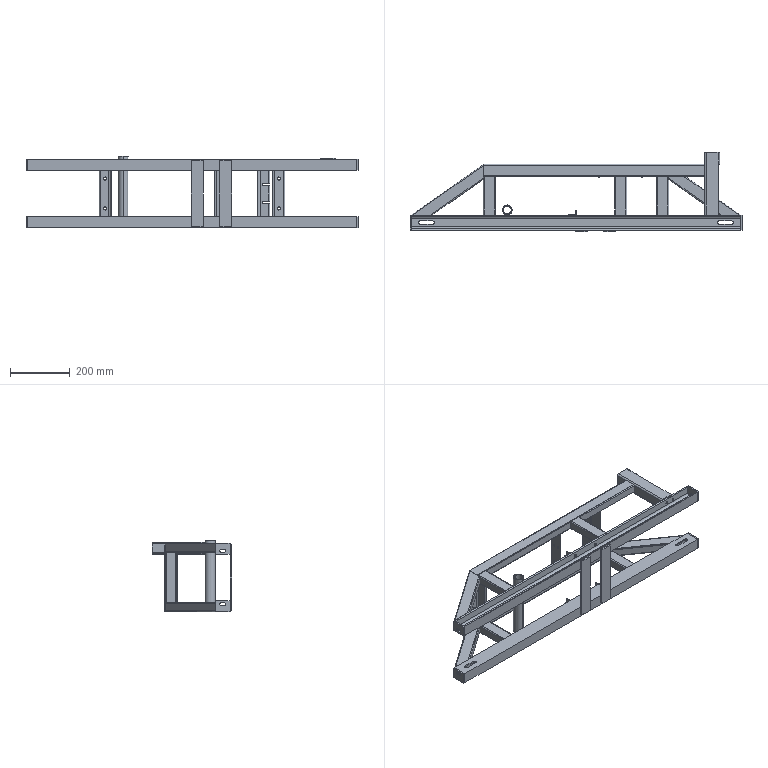Part | SolidWorks | 26 solids | 427 faces | box 1110 x 265 x 240 mm | volume 2389211 mm3 | plane 241 | cylinder 178 | cone 8 | commonest cylinder face diameters 6 x48 1 x36 7 x20 9 x16 10.5 x16 12 x12